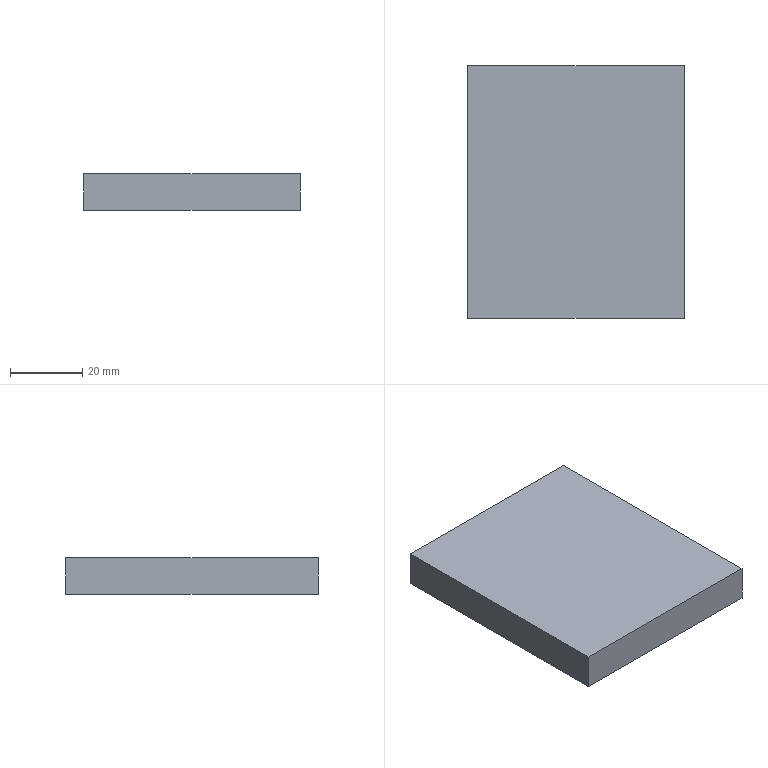Part | SolidWorks | features Extrusion 1 | 1 solid | 6 faces | box 60 x 70 x 10 mm | volume 42000 mm3 | plane 6
STEP:
#1=CARTESIAN_POINT('',(0.,70.,0.));
#2=VERTEX_POINT('',#1);
#3=CARTESIAN_POINT('',(0.,0.,0.));
#4=VERTEX_POINT('',#3);
#5=CARTESIAN_POINT('',(0.,70.,0.));
#6=DIRECTION('',(0.,-1.,0.));
#7=VECTOR('',#6,1000.);
#8=LINE('',#5,#7);
#9=EDGE_CURVE('',#2,#4,#8,.T.);
#10=ORIENTED_EDGE('',*,*,#9,.T.);
#11=CARTESIAN_POINT('',(0.,0.,10.));
#12=VERTEX_POINT('',#11);
#13=CARTESIAN_POINT('',(0.,0.,10.));
#14=DIRECTION('',(0.,0.,-1.));
#15=VECTOR('',#14,1000.);
#16=LINE('',#13,#15);
#17=EDGE_CURVE('',#12,#4,#16,.T.);
#18=ORIENTED_EDGE('',*,*,#17,.F.);
#19=CARTESIAN_POINT('',(0.,70.,10.));
#20=VERTEX_POINT('',#19);
#21=CARTESIAN_POINT('',(0.,70.,10.));
#22=DIRECTION('',(0.,-1.,0.));
#23=VECTOR('',#22,1000.);
#24=LINE('',#21,#23);
#25=EDGE_CURVE('',#20,#12,#24,.T.);
#26=ORIENTED_EDGE('',*,*,#25,.F.);
#27=CARTESIAN_POINT('',(0.,70.,10.));
#28=DIRECTION('',(0.,0.,-1.));
#29=VECTOR('',#28,1000.);
#30=LINE('',#27,#29);
#31=EDGE_CURVE('',#20,#2,#30,.T.);
#32=ORIENTED_EDGE('',*,*,#31,.T.);
#33=EDGE_LOOP('',(#10,#18,#26,#32));
#34=FACE_OUTER_BOUND('',#33,.T.);
#35=CARTESIAN_POINT('',(0.,70.,10.));
#36=DIRECTION('',(1.,0.,0.));
#37=DIRECTION('',(0.,0.,-1.));
#38=AXIS2_PLACEMENT_3D('',#35,#36,#37);
#39=PLANE('',#38);
#40=ADVANCED_FACE('',(#34),#39,.F.);
#41=CARTESIAN_POINT('',(60.,0.,0.));
#42=VERTEX_POINT('',#41);
#43=CARTESIAN_POINT('',(0.,0.,0.));
#44=DIRECTION('',(1.,0.,0.));
#45=VECTOR('',#44,1000.);
#46=LINE('',#43,#45);
#47=EDGE_CURVE('',#4,#42,#46,.T.);
#48=ORIENTED_EDGE('',*,*,#47,.T.);
#49=CARTESIAN_POINT('',(60.,0.,10.));
#50=VERTEX_POINT('',#49);
#51=CARTESIAN_POINT('',(60.,0.,10.));
#52=DIRECTION('',(0.,0.,-1.));
#53=VECTOR('',#52,1000.);
#54=LINE('',#51,#53);
#55=EDGE_CURVE('',#50,#42,#54,.T.);
#56=ORIENTED_EDGE('',*,*,#55,.F.);
#57=CARTESIAN_POINT('',(0.,0.,10.));
#58=DIRECTION('',(1.,0.,0.));
#59=VECTOR('',#58,1000.);
#60=LINE('',#57,#59);
#61=EDGE_CURVE('',#12,#50,#60,.T.);
#62=ORIENTED_EDGE('',*,*,#61,.F.);
#63=ORIENTED_EDGE('',*,*,#17,.T.);
#64=EDGE_LOOP('',(#48,#56,#62,#63));
#65=FACE_OUTER_BOUND('',#64,.T.);
#66=CARTESIAN_POINT('',(0.,0.,10.));
#67=DIRECTION('',(0.,1.,0.));
#68=DIRECTION('',(0.,0.,1.));
#69=AXIS2_PLACEMENT_3D('',#66,#67,#68);
#70=PLANE('',#69);
#71=ADVANCED_FACE('',(#65),#70,.F.);
#72=CARTESIAN_POINT('',(60.,70.,0.));
#73=VERTEX_POINT('',#72);
#74=CARTESIAN_POINT('',(60.,0.,0.));
#75=DIRECTION('',(0.,1.,0.));
#76=VECTOR('',#75,1000.);
#77=LINE('',#74,#76);
#78=EDGE_CURVE('',#42,#73,#77,.T.);
#79=ORIENTED_EDGE('',*,*,#78,.T.);
#80=CARTESIAN_POINT('',(60.,70.,10.));
#81=VERTEX_POINT('',#80);
#82=CARTESIAN_POINT('',(60.,70.,10.));
#83=DIRECTION('',(0.,0.,-1.));
#84=VECTOR('',#83,1000.);
#85=LINE('',#82,#84);
#86=EDGE_CURVE('',#81,#73,#85,.T.);
#87=ORIENTED_EDGE('',*,*,#86,.F.);
#88=CARTESIAN_POINT('',(60.,0.,10.));
#89=DIRECTION('',(0.,1.,0.));
#90=VECTOR('',#89,1000.);
#91=LINE('',#88,#90);
#92=EDGE_CURVE('',#50,#81,#91,.T.);
#93=ORIENTED_EDGE('',*,*,#92,.F.);
#94=ORIENTED_EDGE('',*,*,#55,.T.);
#95=EDGE_LOOP('',(#79,#87,#93,#94));
#96=FACE_OUTER_BOUND('',#95,.T.);
#97=CARTESIAN_POINT('',(60.,0.,10.));
#98=DIRECTION('',(-1.,0.,0.));
#99=DIRECTION('',(0.,0.,1.));
#100=AXIS2_PLACEMENT_3D('',#97,#98,#99);
#101=PLANE('',#100);
#102=ADVANCED_FACE('',(#96),#101,.F.);
#103=CARTESIAN_POINT('',(60.,70.,0.));
#104=DIRECTION('',(-1.,0.,0.));
#105=VECTOR('',#104,1000.);
#106=LINE('',#103,#105);
#107=EDGE_CURVE('',#73,#2,#106,.T.);
#108=ORIENTED_EDGE('',*,*,#107,.T.);
#109=ORIENTED_EDGE('',*,*,#31,.F.);
#110=CARTESIAN_POINT('',(60.,70.,10.));
#111=DIRECTION('',(-1.,0.,0.));
#112=VECTOR('',#111,1000.);
#113=LINE('',#110,#112);
#114=EDGE_CURVE('',#81,#20,#113,.T.);
#115=ORIENTED_EDGE('',*,*,#114,.F.);
#116=ORIENTED_EDGE('',*,*,#86,.T.);
#117=EDGE_LOOP('',(#108,#109,#115,#116));
#118=FACE_OUTER_BOUND('',#117,.T.);
#119=CARTESIAN_POINT('',(60.,70.,10.));
#120=DIRECTION('',(0.,-1.,0.));
#121=DIRECTION('',(0.,0.,-1.));
#122=AXIS2_PLACEMENT_3D('',#119,#120,#121);
#123=PLANE('',#122);
#124=ADVANCED_FACE('',(#118),#123,.F.);
#125=ORIENTED_EDGE('',*,*,#25,.T.);
#126=ORIENTED_EDGE('',*,*,#61,.T.);
#127=ORIENTED_EDGE('',*,*,#92,.T.);
#128=ORIENTED_EDGE('',*,*,#114,.T.);
#129=EDGE_LOOP('',(#125,#126,#127,#128));
#130=FACE_OUTER_BOUND('',#129,.T.);
#131=CARTESIAN_POINT('',(0.,0.,10.));
#132=DIRECTION('',(0.,0.,1.));
#133=DIRECTION('',(1.,0.,0.));
#134=AXIS2_PLACEMENT_3D('',#131,#132,#133);
#135=PLANE('',#134);
#136=ADVANCED_FACE('',(#130),#135,.T.);
#137=ORIENTED_EDGE('',*,*,#9,.F.);
#138=ORIENTED_EDGE('',*,*,#107,.F.);
#139=ORIENTED_EDGE('',*,*,#78,.F.);
#140=ORIENTED_EDGE('',*,*,#47,.F.);
#141=EDGE_LOOP('',(#137,#138,#139,#140));
#142=FACE_OUTER_BOUND('',#141,.T.);
#143=CARTESIAN_POINT('',(0.,0.,0.));
#144=DIRECTION('',(0.,0.,1.));
#145=DIRECTION('',(1.,0.,0.));
#146=AXIS2_PLACEMENT_3D('',#143,#144,#145);
#147=PLANE('',#146);
#148=ADVANCED_FACE('',(#142),#147,.F.);
#149=CLOSED_SHELL('',(#40,#71,#102,#124,#136,#148));
#150=MANIFOLD_SOLID_BREP('',#149);
#151=CARTESIAN_POINT('',(0.,0.,0.));
#152=DIRECTION('',(0.,0.,1.));
#153=DIRECTION('',(1.,0.,0.));
#154=AXIS2_PLACEMENT_3D('',#151,#152,#153);
#155=(LENGTH_UNIT()NAMED_UNIT(*)SI_UNIT(.MILLI.,.METRE.));
#156=UNCERTAINTY_MEASURE_WITH_UNIT(LENGTH_MEASURE(0.00001),#155,'','');
#157=(NAMED_UNIT(*)PLANE_ANGLE_UNIT()SI_UNIT($,.RADIAN.));
#158=(NAMED_UNIT(*)SI_UNIT($,.STERADIAN.)SOLID_ANGLE_UNIT());
#159=(GEOMETRIC_REPRESENTATION_CONTEXT(3)GLOBAL_UNCERTAINTY_ASSIGNED_CONTEXT((#156))GLOBAL_UNIT_ASSIGNED_CONTEXT((#155,#157,#158))REPRESENTATION_CONTEXT('',''));
#160=ADVANCED_BREP_SHAPE_REPRESENTATION('',(#150,#154),#159);